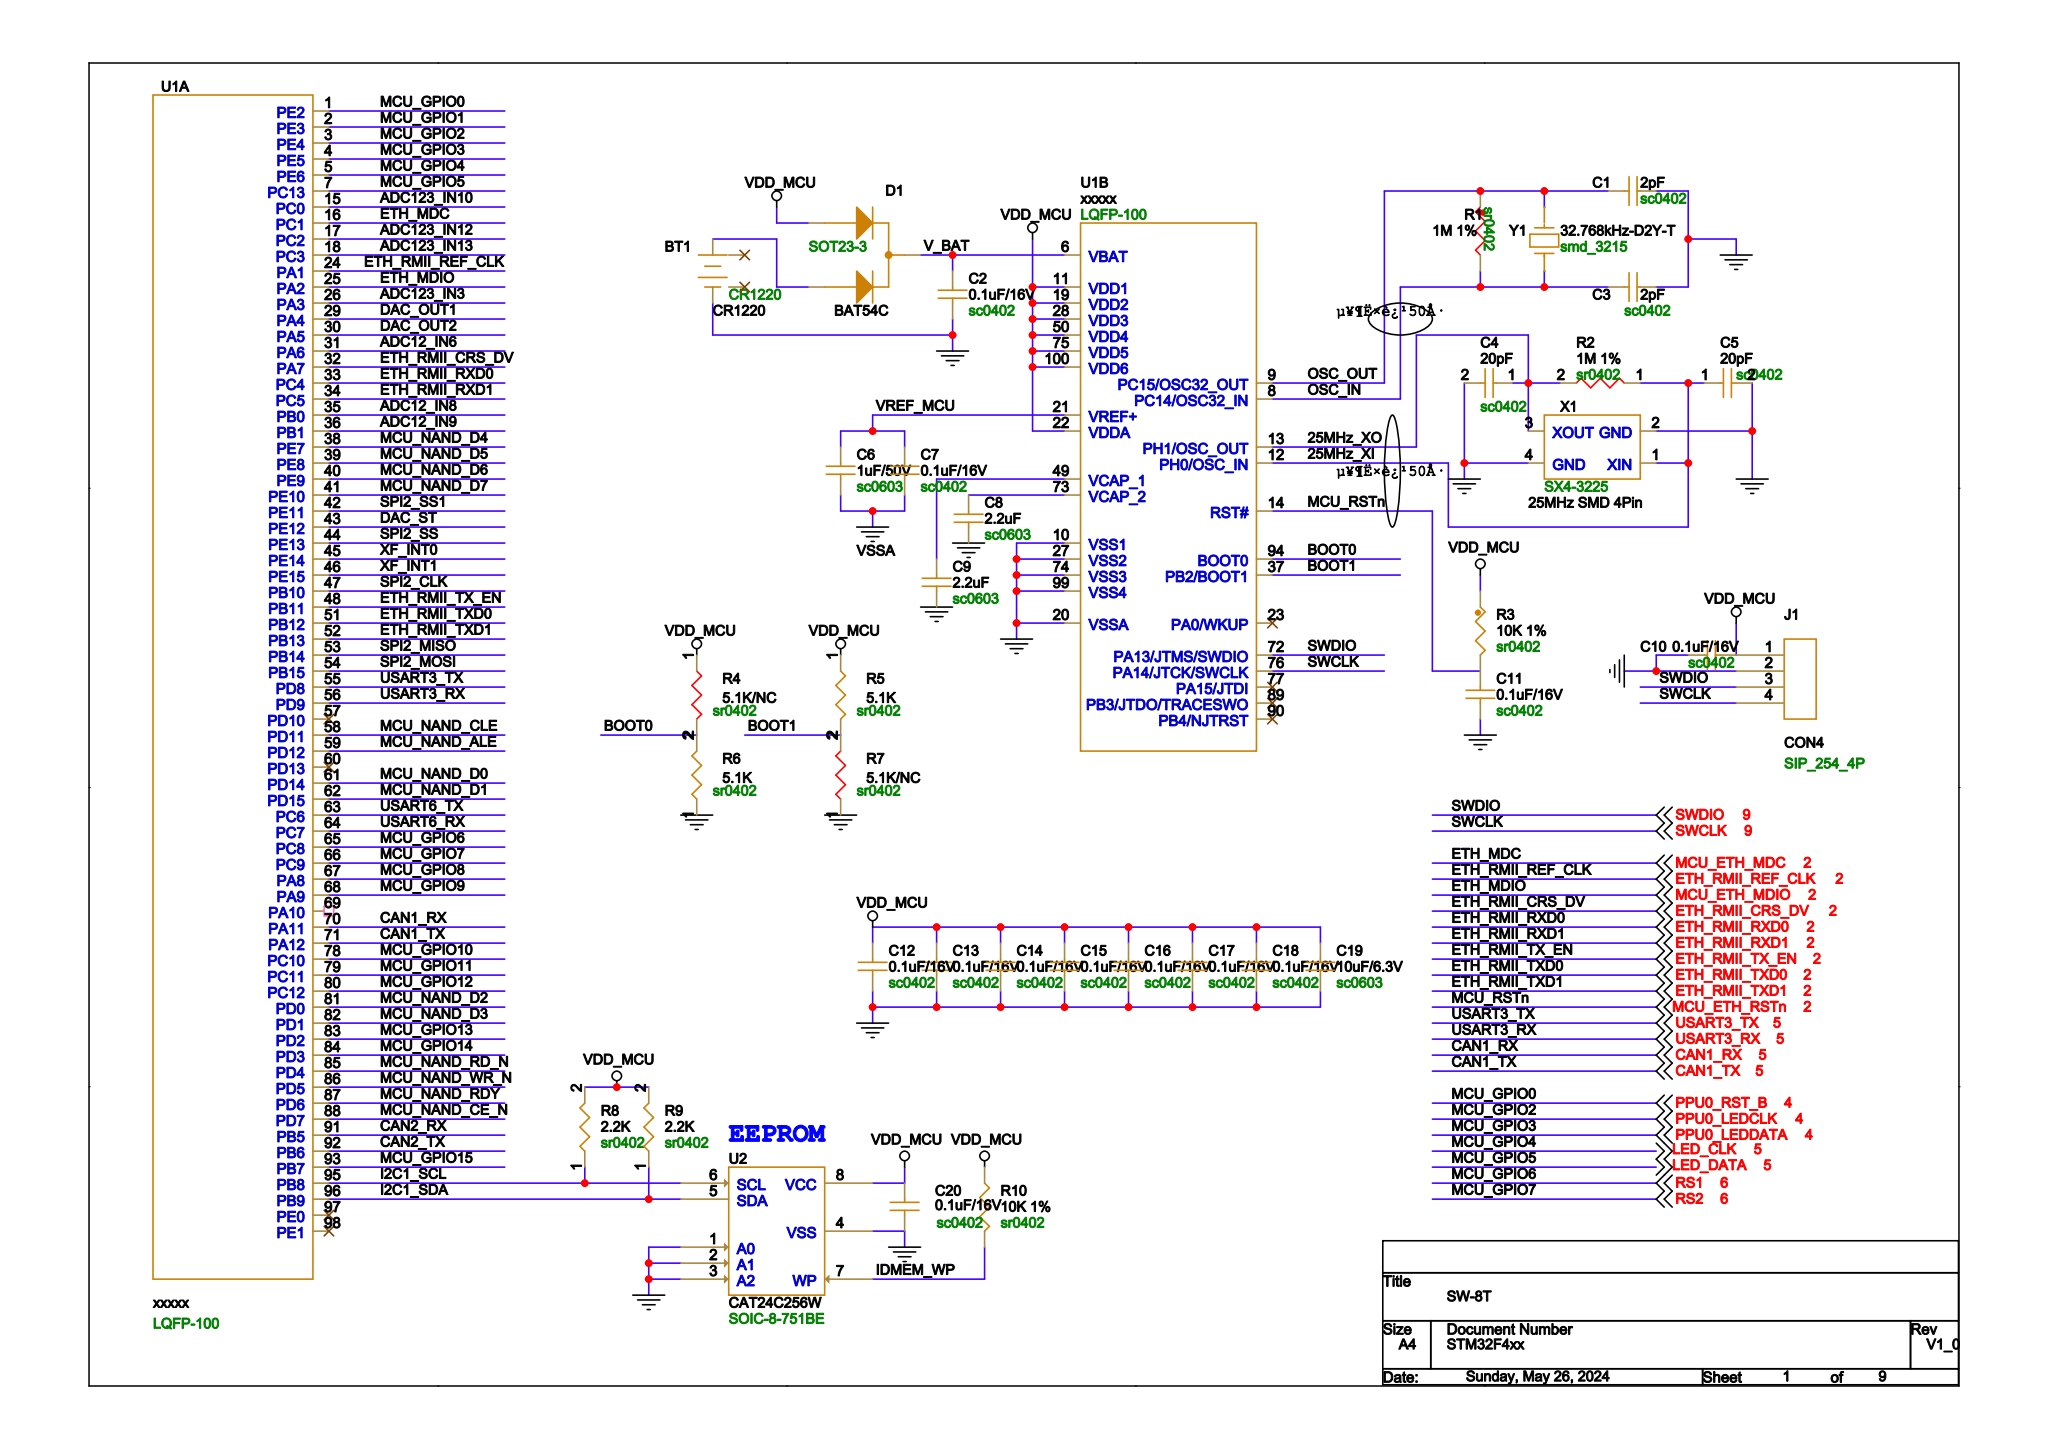Circuit board | Cadence Allegro | 399 parts | 387 nets | one sheet of the schematic
Parts on this sheet (reference | value | footprint):
BT1 | CR1220 | CR1220
C1 | 2pF | SC0402
C2 | 0.1uF/16V | SC0402
C3 | 2pF | SC0402
C4 | 20pF | SC0402
C5 | 20pF | SC0402
C6 | 1uF/50V | SC0603
C7 | 0.1uF/16V | SC0402
C8 | 2.2uF | SC0603
C9 | 2.2uF | SC0603
C10 | 0.1uF/16V | SC0402
C11 | 0.1uF/16V | SC0402
C12 | 0.1uF/16V | SC0402
C13 | 0.1uF/16V | SC0402
C14 | 0.1uF/16V | SC0402
C15 | 0.1uF/16V | SC0402
C16 | 0.1uF/16V | SC0402
C17 | 0.1uF/16V | SC0402
C18 | 0.1uF/16V | SC0402
C19 | 10uF/6.3V | SC0603
C20 | 0.1uF/16V | SC0402
D1 | BAT54C | SOT23-3
J1 | CON4 | SIP_254_4P
R1 | 1M 1% | SR0402
R2 | 1M 1% | SR0402
R3 | 10K 1% | SR0402
R4 | 5.1K/NC | SR0402
R5 | 5.1K | SR0402
R6 | 5.1K | SR0402
R7 | 5.1K/NC | SR0402
R8 | 2.2K | SR0402
R9 | 2.2K | SR0402
R10 | 10K 1% | SR0402
U1 | xxxxx | LQFP-100
U2 | CAT24C256W | SOIC-8-751BE
X1 | 25MHz SMD 4Pin | SX4-3225
Y1 | 32.768kHz-D2Y-T | SMD_3215
Nets of these parts (net: part-pin ...):
GND: BT1-2 C1-1 C2-2 C3-1 C4-2 C5-2 C8-2 C9-2 C10-1 C11-2 C12-2 C13-2 C14-2 C15-2 C16-2 C17-2 C18-2 C19-2 C20-2 J1-2 R6-1 R7-1 U2-1 U2-2 U2-3 U2-4 X1-2 X1-4 U1-10 U1-20 U1-27 U1-74 U1-99
USART3_RX: U1-56
USART3_TX: U1-55
VDD_MCU: C10-2 C12-1 C13-1 C14-1 C15-1 C16-1 C17-1 C18-1 C19-1 C20-1 D1-2 J1-1 R3-1 R4-1 R5-1 R8-2 R9-2 R10-2 U2-8 U1-11 U1-19 U1-22 U1-28 U1-50 U1-75 U1-100
N17778309: BT1-1 D1-1
OSC_OUT: C1-2 R1-1 Y1-2 U1-9
OSC_IN: C3-2 R1-2 Y1-1 U1-8
MCU_ETH_RSTN: C11-1 R3-2 U1-14
V_BAT: C2-1 D1-3 U1-6
VREF_MCU: C6-1 C7-1 U1-21
VSSA: C6-2 C7-2
25MHZ_XO: C4-1 R2-2 X1-3 U1-13
25MHZ_XI: C5-1 R2-1 X1-1 U1-12
N17443317: C8-1 U1-73
N17443310: C9-1 U1-49
CAN1_RX: U1-70
SWDIO: J1-3 U1-72
SWCLK: J1-4 U1-76
IDMEM_WP: R10-1 U2-7
RS2: U1-66
RS1: U1-65
MCU_ETH_MDIO: U1-25
PPU0_RST_B: U1-1
PPU0_LEDCLK: U1-3
PPU0_LEDDATA: U1-4
BOOT0: R4-2 R6-2 U1-94
BOOT1: R5-2 R7-2 U1-37
CAN1_TX: U1-71
I2C1_SCL: R8-1 U2-6 U1-95
I2C1_SDA: R9-1 U2-5 U1-96
ETH_RMII_REF_CLK: U1-24
ADC123_IN3: U1-26
DAC_OUT1: U1-29
DAC_OUT2: U1-30
ADC12_IN6: U1-31
ETH_RMII_CRS_DV: U1-32
MCU_GPIO8: U1-67
MCU_GPIO9: U1-68
ADC12_IN8: U1-35
ADC12_IN9: U1-36
SPI2_CLK: U1-47
ETH_RMII_TX_EN: U1-48
ETH_RMII_TXD0: U1-51
ETH_RMII_TXD1: U1-52
SPI2_MISO: U1-53
SPI2_MOSI: U1-54
CAN2_RX: U1-91
CAN2_TX: U1-92
MCU_GPIO15: U1-93
ADC123_IN10: U1-15
MCU_ETH_MDC: U1-16
MCU_GPIO10: U1-78
MCU_GPIO11: U1-79
MCU_GPIO12: U1-80
LED_DATA: U1-7
ADC123_IN12: U1-17
ADC123_IN13: U1-18
ETH_RMII_RXD0: U1-33
ETH_RMII_RXD1: U1-34
USART6_TX: U1-63
USART6_RX: U1-64
MCU_NAND_D2: U1-81
MCU_NAND_D3: U1-82
MCU_NAND_CLE: U1-58
MCU_NAND_ALE: U1-59
MCU_NAND_D0: U1-61
MCU_NAND_D1: U1-62
MCU_GPIO13: U1-83
MCU_GPIO14: U1-84
MCU_NAND_RD_N: U1-85
MCU_NAND_WR_N: U1-86
MCU_NAND_RDY: U1-87
MCU_NAND_CE_N: U1-88
MCU_NAND_D7: U1-41
SPI2_SS1: U1-42
DAC_ST: U1-43
SPI2_SS: U1-44
XF_INT0: U1-45
XF_INT1: U1-46
MCU_GPIO1: U1-2
LED_CLK: U1-5
MCU_NAND_D4: U1-38
MCU_NAND_D5: U1-39
MCU_NAND_D6: U1-40